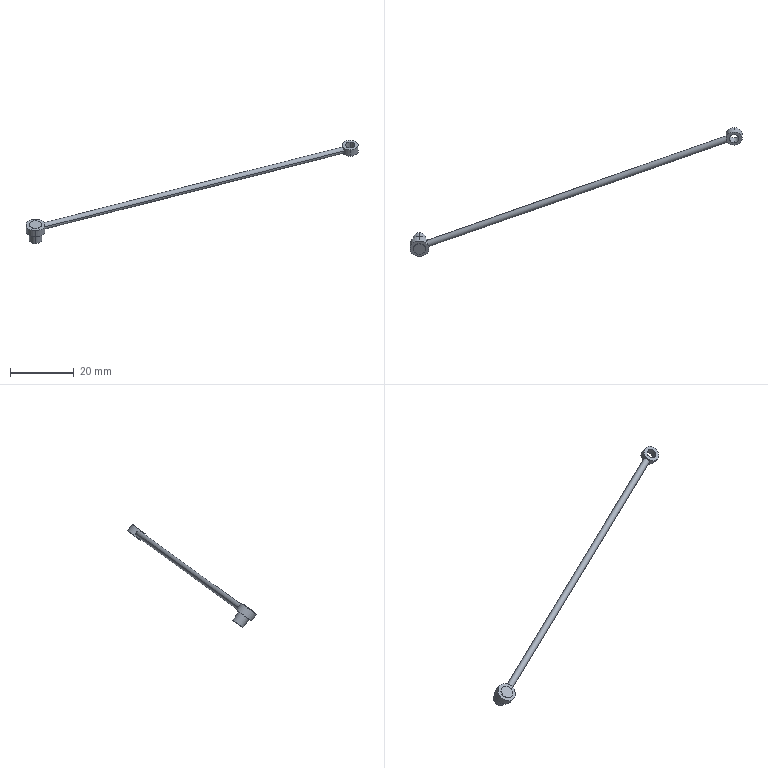Part | STEP file | Completa.sldasm-Part-146_Valor predeterminado | 1 solid | 18 faces | box 104.599 x 40.544 x 32.494 mm | volume 468.209 mm3 | cylinder 12 | plane 6 | commonest cylinder face diameters 4 x4 2 x2 3 x2 5 x2 6 x2